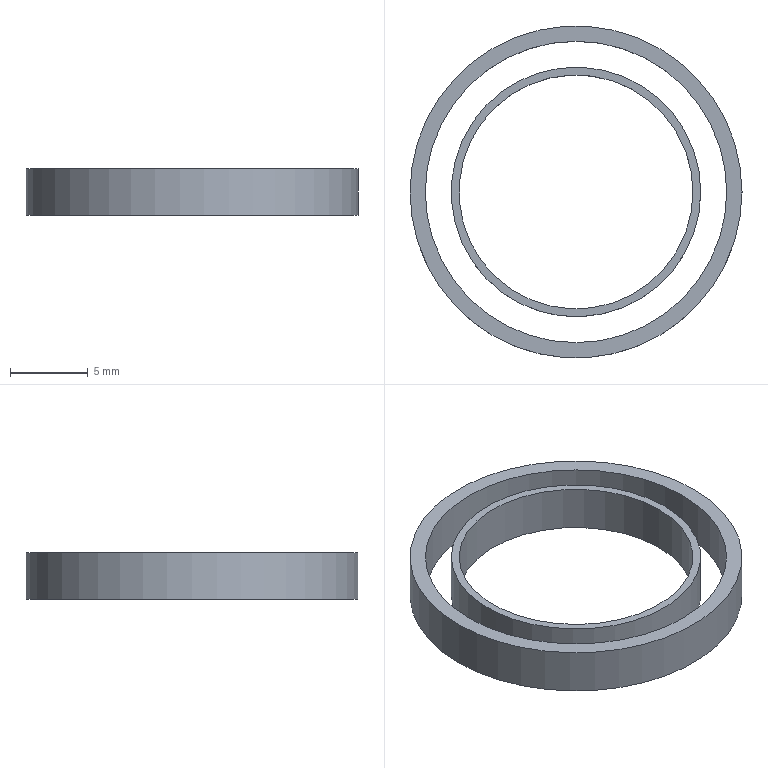Part | NX | features DATUM_CSYS 2, CYLINDER 1, EXTRUDE 1, SKETCH 1 | 2 solids | 8 faces | box 21.29 x 21.29 x 3 mm | volume 261.353 mm3 | cylinder 4 | plane 4 | commonest cylinder face diameters 15 x1 16 x1 19.322 x1 21.29 x1
STEP:
#1=CARTESIAN_POINT('',(10.645,0.,3.));
#2=VERTEX_POINT('',#1);
#3=CARTESIAN_POINT('',(0.,0.,3.));
#4=DIRECTION('',(0.,0.,1.));
#5=DIRECTION('',(1.,0.,0.));
#6=AXIS2_PLACEMENT_3D('',#3,#4,#5);
#7=CIRCLE('',#6,10.645);
#8=EDGE_CURVE('',#2,#2,#7,.T.);
#9=ORIENTED_EDGE('',*,*,#8,.F.);
#10=EDGE_LOOP('',(#9));
#11=FACE_BOUND('',#10,.T.);
#12=CARTESIAN_POINT('',(10.645,0.,0.));
#13=VERTEX_POINT('',#12);
#14=CARTESIAN_POINT('',(0.,0.,0.));
#15=DIRECTION('',(0.,0.,1.));
#16=DIRECTION('',(1.,0.,0.));
#17=AXIS2_PLACEMENT_3D('',#14,#15,#16);
#18=CIRCLE('',#17,10.645);
#19=EDGE_CURVE('',#13,#13,#18,.T.);
#20=ORIENTED_EDGE('',*,*,#19,.T.);
#21=EDGE_LOOP('',(#20));
#22=FACE_BOUND('',#21,.T.);
#23=CARTESIAN_POINT('',(0.,0.,3.));
#24=DIRECTION('',(0.,0.,-1.));
#25=DIRECTION('',(-1.,0.,0.));
#26=AXIS2_PLACEMENT_3D('',#23,#24,#25);
#27=CYLINDRICAL_SURFACE('',#26,10.645);
#28=ADVANCED_FACE('',(#11,#22),#27,.T.);
#29=CARTESIAN_POINT('',(9.661,0.,3.));
#30=VERTEX_POINT('',#29);
#31=CARTESIAN_POINT('',(0.,0.,3.));
#32=DIRECTION('',(0.,0.,1.));
#33=DIRECTION('',(1.,0.,0.));
#34=AXIS2_PLACEMENT_3D('',#31,#32,#33);
#35=CIRCLE('',#34,9.661);
#36=EDGE_CURVE('',#30,#30,#35,.T.);
#37=ORIENTED_EDGE('',*,*,#36,.T.);
#38=EDGE_LOOP('',(#37));
#39=FACE_BOUND('',#38,.T.);
#40=CARTESIAN_POINT('',(9.661,0.,0.));
#41=VERTEX_POINT('',#40);
#42=CARTESIAN_POINT('',(0.,0.,0.));
#43=DIRECTION('',(0.,0.,1.));
#44=DIRECTION('',(1.,0.,0.));
#45=AXIS2_PLACEMENT_3D('',#42,#43,#44);
#46=CIRCLE('',#45,9.661);
#47=EDGE_CURVE('',#41,#41,#46,.T.);
#48=ORIENTED_EDGE('',*,*,#47,.F.);
#49=EDGE_LOOP('',(#48));
#50=FACE_BOUND('',#49,.T.);
#51=CARTESIAN_POINT('',(0.,0.,3.));
#52=DIRECTION('',(0.,0.,-1.));
#53=DIRECTION('',(-1.,0.,0.));
#54=AXIS2_PLACEMENT_3D('',#51,#52,#53);
#55=CYLINDRICAL_SURFACE('',#54,9.661);
#56=ADVANCED_FACE('',(#39,#50),#55,.F.);
#57=ORIENTED_EDGE('',*,*,#8,.T.);
#58=EDGE_LOOP('',(#57));
#59=FACE_BOUND('',#58,.T.);
#60=ORIENTED_EDGE('',*,*,#36,.F.);
#61=EDGE_LOOP('',(#60));
#62=FACE_BOUND('',#61,.T.);
#63=CARTESIAN_POINT('',(0.,0.,3.));
#64=DIRECTION('',(0.,0.,1.));
#65=DIRECTION('',(1.,0.,0.));
#66=AXIS2_PLACEMENT_3D('',#63,#64,#65);
#67=PLANE('',#66);
#68=ADVANCED_FACE('',(#59,#62),#67,.T.);
#69=ORIENTED_EDGE('',*,*,#19,.F.);
#70=EDGE_LOOP('',(#69));
#71=FACE_BOUND('',#70,.T.);
#72=ORIENTED_EDGE('',*,*,#47,.T.);
#73=EDGE_LOOP('',(#72));
#74=FACE_BOUND('',#73,.T.);
#75=CARTESIAN_POINT('',(0.,0.,0.));
#76=DIRECTION('',(0.,0.,1.));
#77=DIRECTION('',(1.,0.,0.));
#78=AXIS2_PLACEMENT_3D('',#75,#76,#77);
#79=PLANE('',#78);
#80=ADVANCED_FACE('',(#71,#74),#79,.F.);
#81=CLOSED_SHELL('',(#28,#56,#68,#80));
#82=MANIFOLD_SOLID_BREP('',#81);
#83=CARTESIAN_POINT('',(8.,0.,3.));
#84=VERTEX_POINT('',#83);
#85=CARTESIAN_POINT('',(0.,0.,3.));
#86=DIRECTION('',(0.,0.,1.));
#87=DIRECTION('',(1.,0.,0.));
#88=AXIS2_PLACEMENT_3D('',#85,#86,#87);
#89=CIRCLE('',#88,8.);
#90=EDGE_CURVE('',#84,#84,#89,.T.);
#91=ORIENTED_EDGE('',*,*,#90,.F.);
#92=EDGE_LOOP('',(#91));
#93=FACE_BOUND('',#92,.T.);
#94=CARTESIAN_POINT('',(8.,0.,0.));
#95=VERTEX_POINT('',#94);
#96=CARTESIAN_POINT('',(0.,0.,0.));
#97=DIRECTION('',(0.,0.,1.));
#98=DIRECTION('',(1.,0.,0.));
#99=AXIS2_PLACEMENT_3D('',#96,#97,#98);
#100=CIRCLE('',#99,8.);
#101=EDGE_CURVE('',#95,#95,#100,.T.);
#102=ORIENTED_EDGE('',*,*,#101,.T.);
#103=EDGE_LOOP('',(#102));
#104=FACE_BOUND('',#103,.T.);
#105=CARTESIAN_POINT('',(0.,0.,3.));
#106=DIRECTION('',(0.,0.,-1.));
#107=DIRECTION('',(-1.,0.,0.));
#108=AXIS2_PLACEMENT_3D('',#105,#106,#107);
#109=CYLINDRICAL_SURFACE('',#108,8.);
#110=ADVANCED_FACE('',(#93,#104),#109,.T.);
#111=CARTESIAN_POINT('',(7.5,0.,3.));
#112=VERTEX_POINT('',#111);
#113=CARTESIAN_POINT('',(0.,0.,3.));
#114=DIRECTION('',(0.,0.,-1.));
#115=DIRECTION('',(1.,0.,0.));
#116=AXIS2_PLACEMENT_3D('',#113,#114,#115);
#117=CIRCLE('',#116,7.5);
#118=EDGE_CURVE('',#112,#112,#117,.T.);
#119=ORIENTED_EDGE('',*,*,#118,.T.);
#120=EDGE_LOOP('',(#119));
#121=FACE_BOUND('',#120,.T.);
#122=ORIENTED_EDGE('',*,*,#90,.T.);
#123=EDGE_LOOP('',(#122));
#124=FACE_BOUND('',#123,.T.);
#125=CARTESIAN_POINT('',(0.,0.,3.));
#126=DIRECTION('',(0.,0.,1.));
#127=DIRECTION('',(1.,0.,0.));
#128=AXIS2_PLACEMENT_3D('',#125,#126,#127);
#129=PLANE('',#128);
#130=ADVANCED_FACE('',(#121,#124),#129,.T.);
#131=CARTESIAN_POINT('',(7.5,0.,0.));
#132=VERTEX_POINT('',#131);
#133=CARTESIAN_POINT('',(0.,0.,0.));
#134=DIRECTION('',(0.,0.,1.));
#135=DIRECTION('',(1.,0.,0.));
#136=AXIS2_PLACEMENT_3D('',#133,#134,#135);
#137=CIRCLE('',#136,7.5);
#138=EDGE_CURVE('',#132,#132,#137,.T.);
#139=ORIENTED_EDGE('',*,*,#138,.T.);
#140=EDGE_LOOP('',(#139));
#141=FACE_BOUND('',#140,.T.);
#142=ORIENTED_EDGE('',*,*,#101,.F.);
#143=EDGE_LOOP('',(#142));
#144=FACE_BOUND('',#143,.T.);
#145=CARTESIAN_POINT('',(0.,0.,0.));
#146=DIRECTION('',(0.,0.,1.));
#147=DIRECTION('',(1.,0.,0.));
#148=AXIS2_PLACEMENT_3D('',#145,#146,#147);
#149=PLANE('',#148);
#150=ADVANCED_FACE('',(#141,#144),#149,.F.);
#151=ORIENTED_EDGE('',*,*,#118,.F.);
#152=EDGE_LOOP('',(#151));
#153=FACE_BOUND('',#152,.T.);
#154=ORIENTED_EDGE('',*,*,#138,.F.);
#155=EDGE_LOOP('',(#154));
#156=FACE_BOUND('',#155,.T.);
#157=CARTESIAN_POINT('',(0.,0.,3.));
#158=DIRECTION('',(0.,0.,-1.));
#159=DIRECTION('',(1.,0.,0.));
#160=AXIS2_PLACEMENT_3D('',#157,#158,#159);
#161=CYLINDRICAL_SURFACE('',#160,7.5);
#162=ADVANCED_FACE('',(#153,#156),#161,.F.);
#163=CLOSED_SHELL('',(#110,#130,#150,#162));
#164=MANIFOLD_SOLID_BREP('',#163);
#165=(LENGTH_UNIT()NAMED_UNIT(*)SI_UNIT(.MILLI.,.METRE.));
#166=UNCERTAINTY_MEASURE_WITH_UNIT(LENGTH_MEASURE(0.00001),#165,'','');
#167=(NAMED_UNIT(*)PLANE_ANGLE_UNIT()SI_UNIT($,.RADIAN.));
#168=(NAMED_UNIT(*)SI_UNIT($,.STERADIAN.)SOLID_ANGLE_UNIT());
#169=(GEOMETRIC_REPRESENTATION_CONTEXT(3)GLOBAL_UNCERTAINTY_ASSIGNED_CONTEXT((#166))GLOBAL_UNIT_ASSIGNED_CONTEXT((#165,#167,#168))REPRESENTATION_CONTEXT('',''));
#170=ADVANCED_BREP_SHAPE_REPRESENTATION('',(#82,#164),#169);